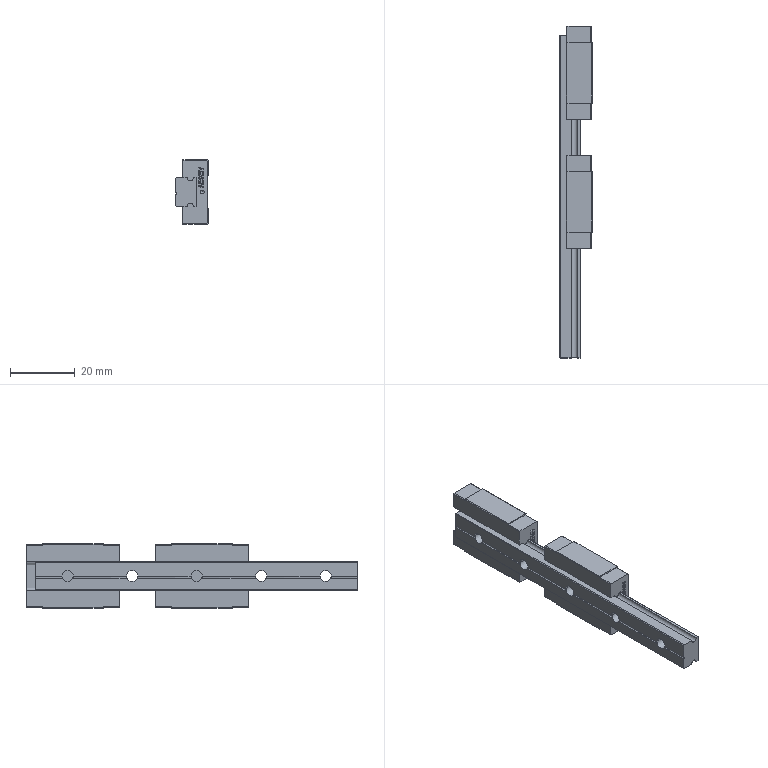Part | SolidWorks | 3 solids | 451 faces | box 10 x 102.865 x 20 mm | volume 11482 mm3 | plane 254 | spline 110 | cylinder 63 | cone 24 | commonest cylinder face diameters 3 x16 0.6 x10 6 x10 2 x9 1.2 x8 3.5 x6